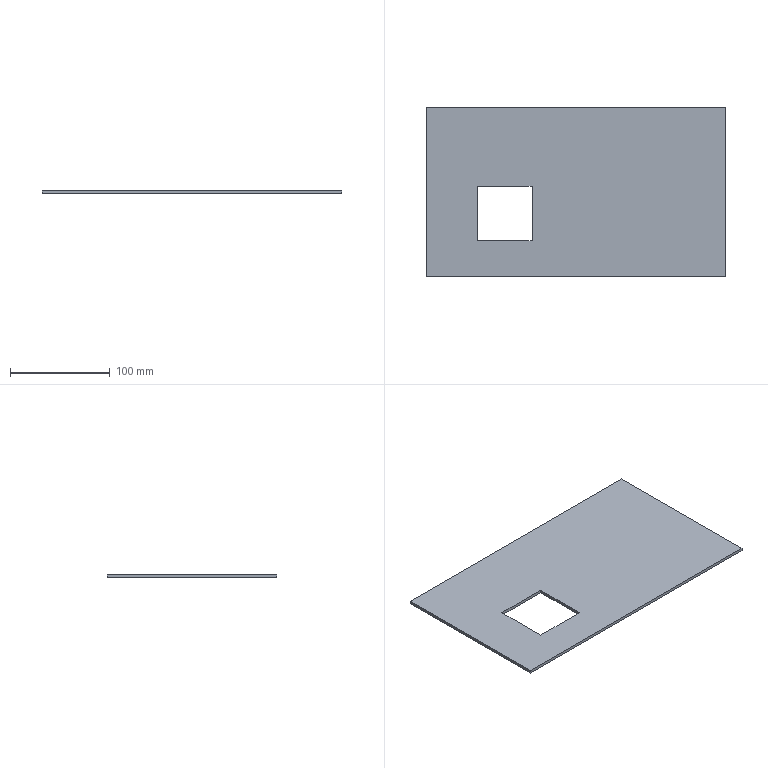Part | SolidWorks | features Cut 1, Extrusion 1 | 1 solid | 10 faces | box 300 x 170 x 3 mm | volume 143925 mm3 | plane 10
STEP:
#1=CARTESIAN_POINT('',(130.,-85.,0.));
#2=VERTEX_POINT('',#1);
#3=CARTESIAN_POINT('',(130.,85.,0.));
#4=VERTEX_POINT('',#3);
#5=CARTESIAN_POINT('',(130.,85.,0.));
#6=DIRECTION('',(0.,1.,0.));
#7=VECTOR('',#6,1000.);
#8=LINE('',#5,#7);
#9=EDGE_CURVE('',#2,#4,#8,.T.);
#10=ORIENTED_EDGE('',*,*,#9,.T.);
#11=CARTESIAN_POINT('',(130.,85.,3.));
#12=VERTEX_POINT('',#11);
#13=CARTESIAN_POINT('',(130.,85.,3.));
#14=DIRECTION('',(0.,0.,-1.));
#15=VECTOR('',#14,1000.);
#16=LINE('',#13,#15);
#17=EDGE_CURVE('',#12,#4,#16,.T.);
#18=ORIENTED_EDGE('',*,*,#17,.F.);
#19=CARTESIAN_POINT('',(130.,-85.,3.));
#20=VERTEX_POINT('',#19);
#21=CARTESIAN_POINT('',(130.,85.,3.));
#22=DIRECTION('',(0.,1.,0.));
#23=VECTOR('',#22,1000.);
#24=LINE('',#21,#23);
#25=EDGE_CURVE('',#20,#12,#24,.T.);
#26=ORIENTED_EDGE('',*,*,#25,.F.);
#27=CARTESIAN_POINT('',(130.,-85.,3.));
#28=DIRECTION('',(0.,0.,-1.));
#29=VECTOR('',#28,1000.);
#30=LINE('',#27,#29);
#31=EDGE_CURVE('',#20,#2,#30,.T.);
#32=ORIENTED_EDGE('',*,*,#31,.T.);
#33=EDGE_LOOP('',(#10,#18,#26,#32));
#34=FACE_OUTER_BOUND('',#33,.T.);
#35=CARTESIAN_POINT('',(130.,85.,3.));
#36=DIRECTION('',(-1.,0.,0.));
#37=DIRECTION('',(0.,0.,1.));
#38=AXIS2_PLACEMENT_3D('',#35,#36,#37);
#39=PLANE('',#38);
#40=ADVANCED_FACE('',(#34),#39,.F.);
#41=CARTESIAN_POINT('',(-170.,85.,0.));
#42=VERTEX_POINT('',#41);
#43=CARTESIAN_POINT('',(-170.,85.,0.));
#44=DIRECTION('',(-1.,0.,0.));
#45=VECTOR('',#44,1000.);
#46=LINE('',#43,#45);
#47=EDGE_CURVE('',#4,#42,#46,.T.);
#48=ORIENTED_EDGE('',*,*,#47,.T.);
#49=CARTESIAN_POINT('',(-170.,85.,3.));
#50=VERTEX_POINT('',#49);
#51=CARTESIAN_POINT('',(-170.,85.,3.));
#52=DIRECTION('',(0.,0.,-1.));
#53=VECTOR('',#52,1000.);
#54=LINE('',#51,#53);
#55=EDGE_CURVE('',#50,#42,#54,.T.);
#56=ORIENTED_EDGE('',*,*,#55,.F.);
#57=CARTESIAN_POINT('',(-170.,85.,3.));
#58=DIRECTION('',(-1.,0.,0.));
#59=VECTOR('',#58,1000.);
#60=LINE('',#57,#59);
#61=EDGE_CURVE('',#12,#50,#60,.T.);
#62=ORIENTED_EDGE('',*,*,#61,.F.);
#63=ORIENTED_EDGE('',*,*,#17,.T.);
#64=EDGE_LOOP('',(#48,#56,#62,#63));
#65=FACE_OUTER_BOUND('',#64,.T.);
#66=CARTESIAN_POINT('',(-170.,85.,3.));
#67=DIRECTION('',(0.,-1.,0.));
#68=DIRECTION('',(0.,0.,-1.));
#69=AXIS2_PLACEMENT_3D('',#66,#67,#68);
#70=PLANE('',#69);
#71=ADVANCED_FACE('',(#65),#70,.F.);
#72=CARTESIAN_POINT('',(-170.,-85.,0.));
#73=VERTEX_POINT('',#72);
#74=CARTESIAN_POINT('',(-170.,85.,0.));
#75=DIRECTION('',(0.,-1.,0.));
#76=VECTOR('',#75,1000.);
#77=LINE('',#74,#76);
#78=EDGE_CURVE('',#42,#73,#77,.T.);
#79=ORIENTED_EDGE('',*,*,#78,.T.);
#80=CARTESIAN_POINT('',(-170.,-85.,3.));
#81=VERTEX_POINT('',#80);
#82=CARTESIAN_POINT('',(-170.,-85.,3.));
#83=DIRECTION('',(0.,0.,-1.));
#84=VECTOR('',#83,1000.);
#85=LINE('',#82,#84);
#86=EDGE_CURVE('',#81,#73,#85,.T.);
#87=ORIENTED_EDGE('',*,*,#86,.F.);
#88=CARTESIAN_POINT('',(-170.,85.,3.));
#89=DIRECTION('',(0.,-1.,0.));
#90=VECTOR('',#89,1000.);
#91=LINE('',#88,#90);
#92=EDGE_CURVE('',#50,#81,#91,.T.);
#93=ORIENTED_EDGE('',*,*,#92,.F.);
#94=ORIENTED_EDGE('',*,*,#55,.T.);
#95=EDGE_LOOP('',(#79,#87,#93,#94));
#96=FACE_OUTER_BOUND('',#95,.T.);
#97=CARTESIAN_POINT('',(-170.,85.,3.));
#98=DIRECTION('',(1.,0.,0.));
#99=DIRECTION('',(0.,0.,-1.));
#100=AXIS2_PLACEMENT_3D('',#97,#98,#99);
#101=PLANE('',#100);
#102=ADVANCED_FACE('',(#96),#101,.F.);
#103=CARTESIAN_POINT('',(-170.,-85.,0.));
#104=DIRECTION('',(1.,0.,0.));
#105=VECTOR('',#104,1000.);
#106=LINE('',#103,#105);
#107=EDGE_CURVE('',#73,#2,#106,.T.);
#108=ORIENTED_EDGE('',*,*,#107,.T.);
#109=ORIENTED_EDGE('',*,*,#31,.F.);
#110=CARTESIAN_POINT('',(-170.,-85.,3.));
#111=DIRECTION('',(1.,0.,0.));
#112=VECTOR('',#111,1000.);
#113=LINE('',#110,#112);
#114=EDGE_CURVE('',#81,#20,#113,.T.);
#115=ORIENTED_EDGE('',*,*,#114,.F.);
#116=ORIENTED_EDGE('',*,*,#86,.T.);
#117=EDGE_LOOP('',(#108,#109,#115,#116));
#118=FACE_OUTER_BOUND('',#117,.T.);
#119=CARTESIAN_POINT('',(-170.,-85.,3.));
#120=DIRECTION('',(0.,1.,0.));
#121=DIRECTION('',(0.,0.,1.));
#122=AXIS2_PLACEMENT_3D('',#119,#120,#121);
#123=PLANE('',#122);
#124=ADVANCED_FACE('',(#118),#123,.F.);
#125=CARTESIAN_POINT('',(-119.,-49.,3.));
#126=VERTEX_POINT('',#125);
#127=CARTESIAN_POINT('',(-64.,-49.,3.));
#128=VERTEX_POINT('',#127);
#129=CARTESIAN_POINT('',(0.,-49.,3.));
#130=DIRECTION('',(1.,0.,0.));
#131=VECTOR('',#130,1000.);
#132=LINE('',#129,#131);
#133=EDGE_CURVE('',#126,#128,#132,.T.);
#134=ORIENTED_EDGE('',*,*,#133,.F.);
#135=CARTESIAN_POINT('',(-119.,6.,3.));
#136=VERTEX_POINT('',#135);
#137=CARTESIAN_POINT('',(-119.,0.,3.));
#138=DIRECTION('',(0.,-1.,0.));
#139=VECTOR('',#138,1000.);
#140=LINE('',#137,#139);
#141=EDGE_CURVE('',#136,#126,#140,.T.);
#142=ORIENTED_EDGE('',*,*,#141,.F.);
#143=CARTESIAN_POINT('',(-64.,6.,3.));
#144=VERTEX_POINT('',#143);
#145=CARTESIAN_POINT('',(0.,6.,3.));
#146=DIRECTION('',(-1.,0.,0.));
#147=VECTOR('',#146,1000.);
#148=LINE('',#145,#147);
#149=EDGE_CURVE('',#144,#136,#148,.T.);
#150=ORIENTED_EDGE('',*,*,#149,.F.);
#151=CARTESIAN_POINT('',(-64.,0.,3.));
#152=DIRECTION('',(0.,1.,0.));
#153=VECTOR('',#152,1000.);
#154=LINE('',#151,#153);
#155=EDGE_CURVE('',#128,#144,#154,.T.);
#156=ORIENTED_EDGE('',*,*,#155,.F.);
#157=EDGE_LOOP('',(#134,#142,#150,#156));
#158=FACE_BOUND('',#157,.T.);
#159=ORIENTED_EDGE('',*,*,#25,.T.);
#160=ORIENTED_EDGE('',*,*,#61,.T.);
#161=ORIENTED_EDGE('',*,*,#92,.T.);
#162=ORIENTED_EDGE('',*,*,#114,.T.);
#163=EDGE_LOOP('',(#159,#160,#161,#162));
#164=FACE_OUTER_BOUND('',#163,.T.);
#165=CARTESIAN_POINT('',(0.,0.,3.));
#166=DIRECTION('',(0.,0.,1.));
#167=DIRECTION('',(1.,0.,0.));
#168=AXIS2_PLACEMENT_3D('',#165,#166,#167);
#169=PLANE('',#168);
#170=ADVANCED_FACE('',(#158,#164),#169,.T.);
#171=CARTESIAN_POINT('',(-119.,-49.,0.));
#172=VERTEX_POINT('',#171);
#173=CARTESIAN_POINT('',(-119.,6.,0.));
#174=VERTEX_POINT('',#173);
#175=CARTESIAN_POINT('',(-119.,-49.,0.));
#176=DIRECTION('',(0.,1.,0.));
#177=VECTOR('',#176,1000.);
#178=LINE('',#175,#177);
#179=EDGE_CURVE('',#172,#174,#178,.T.);
#180=ORIENTED_EDGE('',*,*,#179,.F.);
#181=CARTESIAN_POINT('',(-64.,-49.,0.));
#182=VERTEX_POINT('',#181);
#183=CARTESIAN_POINT('',(-64.,-49.,0.));
#184=DIRECTION('',(-1.,0.,0.));
#185=VECTOR('',#184,1000.);
#186=LINE('',#183,#185);
#187=EDGE_CURVE('',#182,#172,#186,.T.);
#188=ORIENTED_EDGE('',*,*,#187,.F.);
#189=CARTESIAN_POINT('',(-64.,6.,0.));
#190=VERTEX_POINT('',#189);
#191=CARTESIAN_POINT('',(-64.,6.,0.));
#192=DIRECTION('',(0.,-1.,0.));
#193=VECTOR('',#192,1000.);
#194=LINE('',#191,#193);
#195=EDGE_CURVE('',#190,#182,#194,.T.);
#196=ORIENTED_EDGE('',*,*,#195,.F.);
#197=CARTESIAN_POINT('',(-119.,6.,0.));
#198=DIRECTION('',(1.,0.,0.));
#199=VECTOR('',#198,1000.);
#200=LINE('',#197,#199);
#201=EDGE_CURVE('',#174,#190,#200,.T.);
#202=ORIENTED_EDGE('',*,*,#201,.F.);
#203=EDGE_LOOP('',(#180,#188,#196,#202));
#204=FACE_BOUND('',#203,.T.);
#205=ORIENTED_EDGE('',*,*,#9,.F.);
#206=ORIENTED_EDGE('',*,*,#107,.F.);
#207=ORIENTED_EDGE('',*,*,#78,.F.);
#208=ORIENTED_EDGE('',*,*,#47,.F.);
#209=EDGE_LOOP('',(#205,#206,#207,#208));
#210=FACE_OUTER_BOUND('',#209,.T.);
#211=CARTESIAN_POINT('',(0.,0.,0.));
#212=DIRECTION('',(0.,0.,1.));
#213=DIRECTION('',(1.,0.,0.));
#214=AXIS2_PLACEMENT_3D('',#211,#212,#213);
#215=PLANE('',#214);
#216=ADVANCED_FACE('',(#204,#210),#215,.F.);
#217=ORIENTED_EDGE('',*,*,#133,.T.);
#218=CARTESIAN_POINT('',(-64.,-49.,40.5));
#219=DIRECTION('',(0.,0.,-1.));
#220=VECTOR('',#219,1000.);
#221=LINE('',#218,#220);
#222=EDGE_CURVE('',#128,#182,#221,.T.);
#223=ORIENTED_EDGE('',*,*,#222,.T.);
#224=ORIENTED_EDGE('',*,*,#187,.T.);
#225=CARTESIAN_POINT('',(-119.,-49.,40.5));
#226=DIRECTION('',(0.,0.,-1.));
#227=VECTOR('',#226,1000.);
#228=LINE('',#225,#227);
#229=EDGE_CURVE('',#126,#172,#228,.T.);
#230=ORIENTED_EDGE('',*,*,#229,.F.);
#231=EDGE_LOOP('',(#217,#223,#224,#230));
#232=FACE_OUTER_BOUND('',#231,.T.);
#233=CARTESIAN_POINT('',(-64.,-49.,40.5));
#234=DIRECTION('',(0.,-1.,0.));
#235=DIRECTION('',(0.,0.,-1.));
#236=AXIS2_PLACEMENT_3D('',#233,#234,#235);
#237=PLANE('',#236);
#238=ADVANCED_FACE('',(#232),#237,.F.);
#239=ORIENTED_EDGE('',*,*,#155,.T.);
#240=CARTESIAN_POINT('',(-64.,6.,40.5));
#241=DIRECTION('',(0.,0.,-1.));
#242=VECTOR('',#241,1000.);
#243=LINE('',#240,#242);
#244=EDGE_CURVE('',#144,#190,#243,.T.);
#245=ORIENTED_EDGE('',*,*,#244,.T.);
#246=ORIENTED_EDGE('',*,*,#195,.T.);
#247=ORIENTED_EDGE('',*,*,#222,.F.);
#248=EDGE_LOOP('',(#239,#245,#246,#247));
#249=FACE_OUTER_BOUND('',#248,.T.);
#250=CARTESIAN_POINT('',(-64.,6.,40.5));
#251=DIRECTION('',(1.,0.,0.));
#252=DIRECTION('',(0.,0.,-1.));
#253=AXIS2_PLACEMENT_3D('',#250,#251,#252);
#254=PLANE('',#253);
#255=ADVANCED_FACE('',(#249),#254,.F.);
#256=ORIENTED_EDGE('',*,*,#149,.T.);
#257=CARTESIAN_POINT('',(-119.,6.,40.5));
#258=DIRECTION('',(0.,0.,-1.));
#259=VECTOR('',#258,1000.);
#260=LINE('',#257,#259);
#261=EDGE_CURVE('',#136,#174,#260,.T.);
#262=ORIENTED_EDGE('',*,*,#261,.T.);
#263=ORIENTED_EDGE('',*,*,#201,.T.);
#264=ORIENTED_EDGE('',*,*,#244,.F.);
#265=EDGE_LOOP('',(#256,#262,#263,#264));
#266=FACE_OUTER_BOUND('',#265,.T.);
#267=CARTESIAN_POINT('',(-119.,6.,40.5));
#268=DIRECTION('',(0.,1.,0.));
#269=DIRECTION('',(0.,0.,1.));
#270=AXIS2_PLACEMENT_3D('',#267,#268,#269);
#271=PLANE('',#270);
#272=ADVANCED_FACE('',(#266),#271,.F.);
#273=ORIENTED_EDGE('',*,*,#141,.T.);
#274=ORIENTED_EDGE('',*,*,#229,.T.);
#275=ORIENTED_EDGE('',*,*,#179,.T.);
#276=ORIENTED_EDGE('',*,*,#261,.F.);
#277=EDGE_LOOP('',(#273,#274,#275,#276));
#278=FACE_OUTER_BOUND('',#277,.T.);
#279=CARTESIAN_POINT('',(-119.,-49.,40.5));
#280=DIRECTION('',(-1.,0.,0.));
#281=DIRECTION('',(0.,0.,1.));
#282=AXIS2_PLACEMENT_3D('',#279,#280,#281);
#283=PLANE('',#282);
#284=ADVANCED_FACE('',(#278),#283,.F.);
#285=CLOSED_SHELL('',(#40,#71,#102,#124,#170,#216,#238,#255,#272,#284));
#286=MANIFOLD_SOLID_BREP('',#285);
#287=CARTESIAN_POINT('',(0.,0.,0.));
#288=DIRECTION('',(0.,0.,1.));
#289=DIRECTION('',(1.,0.,0.));
#290=AXIS2_PLACEMENT_3D('',#287,#288,#289);
#291=(LENGTH_UNIT()NAMED_UNIT(*)SI_UNIT(.MILLI.,.METRE.));
#292=UNCERTAINTY_MEASURE_WITH_UNIT(LENGTH_MEASURE(0.00001),#291,'','');
#293=(NAMED_UNIT(*)PLANE_ANGLE_UNIT()SI_UNIT($,.RADIAN.));
#294=(NAMED_UNIT(*)SI_UNIT($,.STERADIAN.)SOLID_ANGLE_UNIT());
#295=(GEOMETRIC_REPRESENTATION_CONTEXT(3)GLOBAL_UNCERTAINTY_ASSIGNED_CONTEXT((#292))GLOBAL_UNIT_ASSIGNED_CONTEXT((#291,#293,#294))REPRESENTATION_CONTEXT('',''));
#296=ADVANCED_BREP_SHAPE_REPRESENTATION('',(#286,#290),#295);